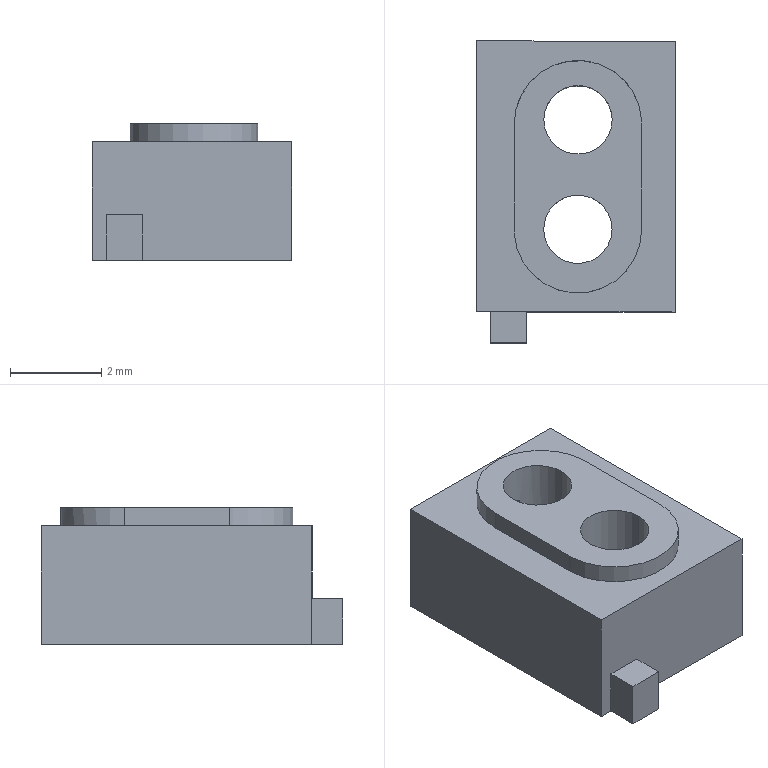Part | Creo | 1 solid | 25 faces | volume 52.759 mm3 | plane 19 | cylinder 6 | commonest cylinder face diameters 1.5 x4 2.8 x2